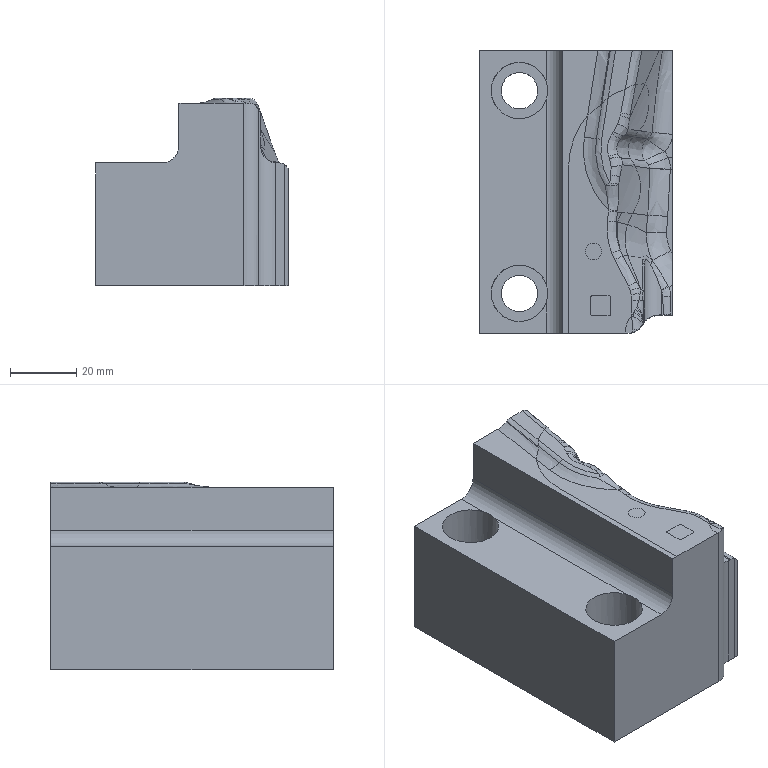Part | STEP file | 1 solid | 123 faces | box 58 x 85.001 x 56.5 mm | volume 200915 mm3 | spline 88 | plane 21 | cylinder 13 | sphere 1 | commonest cylinder face diameters 6 x3 10 x3 11 x2 12 x2 17 x2 14 x1